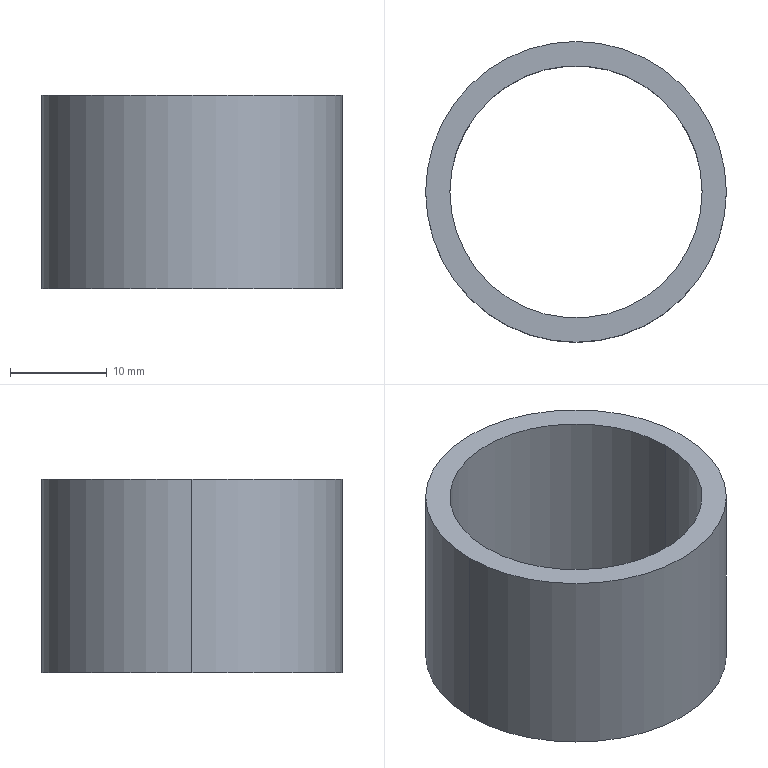Part | STEP file | Pitch ring | 1 solid | 6 faces | box 31 x 31 x 20 mm | volume 4477 mm3 | cylinder 4 | plane 2 | commonest cylinder face diameters 26 x2 31 x2
STEP:
#1=CARTESIAN_POINT('',(-13.,0.,-10.));
#2=VERTEX_POINT('',#1);
#3=CARTESIAN_POINT('',(13.,0.,-10.));
#4=VERTEX_POINT('',#3);
#5=CARTESIAN_POINT('',(0.,0.,-10.));
#6=DIRECTION('',(0.,0.,1.));
#7=DIRECTION('',(1.,0.,0.));
#8=AXIS2_PLACEMENT_3D('',#5,#6,#7);
#9=CIRCLE('',#8,13.);
#10=EDGE_CURVE('',#2,#4,#9,.T.);
#11=ORIENTED_EDGE('',*,*,#10,.F.);
#12=CARTESIAN_POINT('',(-13.,0.,10.));
#13=VERTEX_POINT('',#12);
#14=CARTESIAN_POINT('',(-13.,0.,-10.));
#15=DIRECTION('',(0.,0.,1.));
#16=VECTOR('',#15,1000.);
#17=LINE('',#14,#16);
#18=EDGE_CURVE('',#2,#13,#17,.T.);
#19=ORIENTED_EDGE('',*,*,#18,.T.);
#20=CARTESIAN_POINT('',(13.,0.,10.));
#21=VERTEX_POINT('',#20);
#22=CARTESIAN_POINT('',(0.,0.,10.));
#23=DIRECTION('',(0.,0.,1.));
#24=DIRECTION('',(1.,0.,0.));
#25=AXIS2_PLACEMENT_3D('',#22,#23,#24);
#26=CIRCLE('',#25,13.);
#27=EDGE_CURVE('',#13,#21,#26,.T.);
#28=ORIENTED_EDGE('',*,*,#27,.T.);
#29=CARTESIAN_POINT('',(13.,0.,-10.));
#30=DIRECTION('',(0.,0.,1.));
#31=VECTOR('',#30,1000.);
#32=LINE('',#29,#31);
#33=EDGE_CURVE('',#4,#21,#32,.T.);
#34=ORIENTED_EDGE('',*,*,#33,.F.);
#35=EDGE_LOOP('',(#11,#19,#28,#34));
#36=FACE_OUTER_BOUND('',#35,.T.);
#37=CARTESIAN_POINT('',(0.,0.,-10.));
#38=DIRECTION('',(0.,0.,1.));
#39=DIRECTION('',(1.,0.,0.));
#40=AXIS2_PLACEMENT_3D('',#37,#38,#39);
#41=CYLINDRICAL_SURFACE('',#40,13.);
#42=ADVANCED_FACE('',(#36),#41,.F.);
#43=CARTESIAN_POINT('',(15.5,0.,-10.));
#44=VERTEX_POINT('',#43);
#45=CARTESIAN_POINT('',(-15.5,0.,-10.));
#46=VERTEX_POINT('',#45);
#47=CARTESIAN_POINT('',(0.,0.,-10.));
#48=DIRECTION('',(0.,0.,1.));
#49=DIRECTION('',(1.,0.,0.));
#50=AXIS2_PLACEMENT_3D('',#47,#48,#49);
#51=CIRCLE('',#50,15.5);
#52=EDGE_CURVE('',#44,#46,#51,.T.);
#53=ORIENTED_EDGE('',*,*,#52,.T.);
#54=CARTESIAN_POINT('',(-15.5,0.,10.));
#55=VERTEX_POINT('',#54);
#56=CARTESIAN_POINT('',(-15.5,0.,-10.));
#57=DIRECTION('',(0.,0.,1.));
#58=VECTOR('',#57,1000.);
#59=LINE('',#56,#58);
#60=EDGE_CURVE('',#46,#55,#59,.T.);
#61=ORIENTED_EDGE('',*,*,#60,.T.);
#62=CARTESIAN_POINT('',(15.5,0.,10.));
#63=VERTEX_POINT('',#62);
#64=CARTESIAN_POINT('',(0.,0.,10.));
#65=DIRECTION('',(0.,0.,1.));
#66=DIRECTION('',(1.,0.,0.));
#67=AXIS2_PLACEMENT_3D('',#64,#65,#66);
#68=CIRCLE('',#67,15.5);
#69=EDGE_CURVE('',#63,#55,#68,.T.);
#70=ORIENTED_EDGE('',*,*,#69,.F.);
#71=CARTESIAN_POINT('',(15.5,0.,-10.));
#72=DIRECTION('',(0.,0.,1.));
#73=VECTOR('',#72,1000.);
#74=LINE('',#71,#73);
#75=EDGE_CURVE('',#44,#63,#74,.T.);
#76=ORIENTED_EDGE('',*,*,#75,.F.);
#77=EDGE_LOOP('',(#53,#61,#70,#76));
#78=FACE_OUTER_BOUND('',#77,.T.);
#79=CARTESIAN_POINT('',(0.,0.,-10.));
#80=DIRECTION('',(0.,0.,1.));
#81=DIRECTION('',(1.,0.,0.));
#82=AXIS2_PLACEMENT_3D('',#79,#80,#81);
#83=CYLINDRICAL_SURFACE('',#82,15.5);
#84=ADVANCED_FACE('',(#78),#83,.T.);
#85=ORIENTED_EDGE('',*,*,#60,.F.);
#86=CARTESIAN_POINT('',(0.,0.,-10.));
#87=DIRECTION('',(0.,0.,1.));
#88=DIRECTION('',(1.,0.,0.));
#89=AXIS2_PLACEMENT_3D('',#86,#87,#88);
#90=CIRCLE('',#89,15.5);
#91=EDGE_CURVE('',#46,#44,#90,.T.);
#92=ORIENTED_EDGE('',*,*,#91,.T.);
#93=ORIENTED_EDGE('',*,*,#75,.T.);
#94=CARTESIAN_POINT('',(0.,0.,10.));
#95=DIRECTION('',(0.,0.,1.));
#96=DIRECTION('',(1.,0.,0.));
#97=AXIS2_PLACEMENT_3D('',#94,#95,#96);
#98=CIRCLE('',#97,15.5);
#99=EDGE_CURVE('',#55,#63,#98,.T.);
#100=ORIENTED_EDGE('',*,*,#99,.F.);
#101=EDGE_LOOP('',(#85,#92,#93,#100));
#102=FACE_OUTER_BOUND('',#101,.T.);
#103=CARTESIAN_POINT('',(0.,0.,-10.));
#104=DIRECTION('',(0.,0.,1.));
#105=DIRECTION('',(1.,0.,0.));
#106=AXIS2_PLACEMENT_3D('',#103,#104,#105);
#107=CYLINDRICAL_SURFACE('',#106,15.5);
#108=ADVANCED_FACE('',(#102),#107,.T.);
#109=CARTESIAN_POINT('',(0.,0.,-10.));
#110=DIRECTION('',(0.,0.,1.));
#111=DIRECTION('',(1.,0.,0.));
#112=AXIS2_PLACEMENT_3D('',#109,#110,#111);
#113=CIRCLE('',#112,13.);
#114=EDGE_CURVE('',#4,#2,#113,.T.);
#115=ORIENTED_EDGE('',*,*,#114,.T.);
#116=ORIENTED_EDGE('',*,*,#10,.T.);
#117=EDGE_LOOP('',(#115,#116));
#118=FACE_BOUND('',#117,.T.);
#119=ORIENTED_EDGE('',*,*,#52,.F.);
#120=ORIENTED_EDGE('',*,*,#91,.F.);
#121=EDGE_LOOP('',(#119,#120));
#122=FACE_OUTER_BOUND('',#121,.T.);
#123=CARTESIAN_POINT('',(15.5,0.,-10.));
#124=DIRECTION('',(0.,0.,-1.));
#125=DIRECTION('',(-1.,0.,0.));
#126=AXIS2_PLACEMENT_3D('',#123,#124,#125);
#127=PLANE('',#126);
#128=ADVANCED_FACE('',(#118,#122),#127,.T.);
#129=ORIENTED_EDGE('',*,*,#18,.F.);
#130=ORIENTED_EDGE('',*,*,#114,.F.);
#131=ORIENTED_EDGE('',*,*,#33,.T.);
#132=CARTESIAN_POINT('',(0.,0.,10.));
#133=DIRECTION('',(0.,0.,1.));
#134=DIRECTION('',(1.,0.,0.));
#135=AXIS2_PLACEMENT_3D('',#132,#133,#134);
#136=CIRCLE('',#135,13.);
#137=EDGE_CURVE('',#21,#13,#136,.T.);
#138=ORIENTED_EDGE('',*,*,#137,.T.);
#139=EDGE_LOOP('',(#129,#130,#131,#138));
#140=FACE_OUTER_BOUND('',#139,.T.);
#141=CARTESIAN_POINT('',(0.,0.,-10.));
#142=DIRECTION('',(0.,0.,1.));
#143=DIRECTION('',(1.,0.,0.));
#144=AXIS2_PLACEMENT_3D('',#141,#142,#143);
#145=CYLINDRICAL_SURFACE('',#144,13.);
#146=ADVANCED_FACE('',(#140),#145,.F.);
#147=ORIENTED_EDGE('',*,*,#69,.T.);
#148=ORIENTED_EDGE('',*,*,#99,.T.);
#149=EDGE_LOOP('',(#147,#148));
#150=FACE_OUTER_BOUND('',#149,.T.);
#151=ORIENTED_EDGE('',*,*,#137,.F.);
#152=ORIENTED_EDGE('',*,*,#27,.F.);
#153=EDGE_LOOP('',(#151,#152));
#154=FACE_BOUND('',#153,.T.);
#155=CARTESIAN_POINT('',(13.,0.,10.));
#156=DIRECTION('',(0.,0.,1.));
#157=DIRECTION('',(1.,0.,0.));
#158=AXIS2_PLACEMENT_3D('',#155,#156,#157);
#159=PLANE('',#158);
#160=ADVANCED_FACE('',(#150,#154),#159,.T.);
#161=CLOSED_SHELL('',(#42,#84,#108,#128,#146,#160));
#162=MANIFOLD_SOLID_BREP('',#161);
#163=CARTESIAN_POINT('',(0.,0.,0.));
#164=DIRECTION('',(0.,0.,1.));
#165=DIRECTION('',(1.,0.,0.));
#166=AXIS2_PLACEMENT_3D('',#163,#164,#165);
#167=(LENGTH_UNIT()NAMED_UNIT(*)SI_UNIT(.MILLI.,.METRE.));
#168=UNCERTAINTY_MEASURE_WITH_UNIT(LENGTH_MEASURE(0.00001),#167,'','');
#169=(NAMED_UNIT(*)PLANE_ANGLE_UNIT()SI_UNIT($,.RADIAN.));
#170=(NAMED_UNIT(*)SI_UNIT($,.STERADIAN.)SOLID_ANGLE_UNIT());
#171=(GEOMETRIC_REPRESENTATION_CONTEXT(3)GLOBAL_UNCERTAINTY_ASSIGNED_CONTEXT((#168))GLOBAL_UNIT_ASSIGNED_CONTEXT((#167,#169,#170))REPRESENTATION_CONTEXT('',''));
#172=ADVANCED_BREP_SHAPE_REPRESENTATION('',(#162,#166),#171);